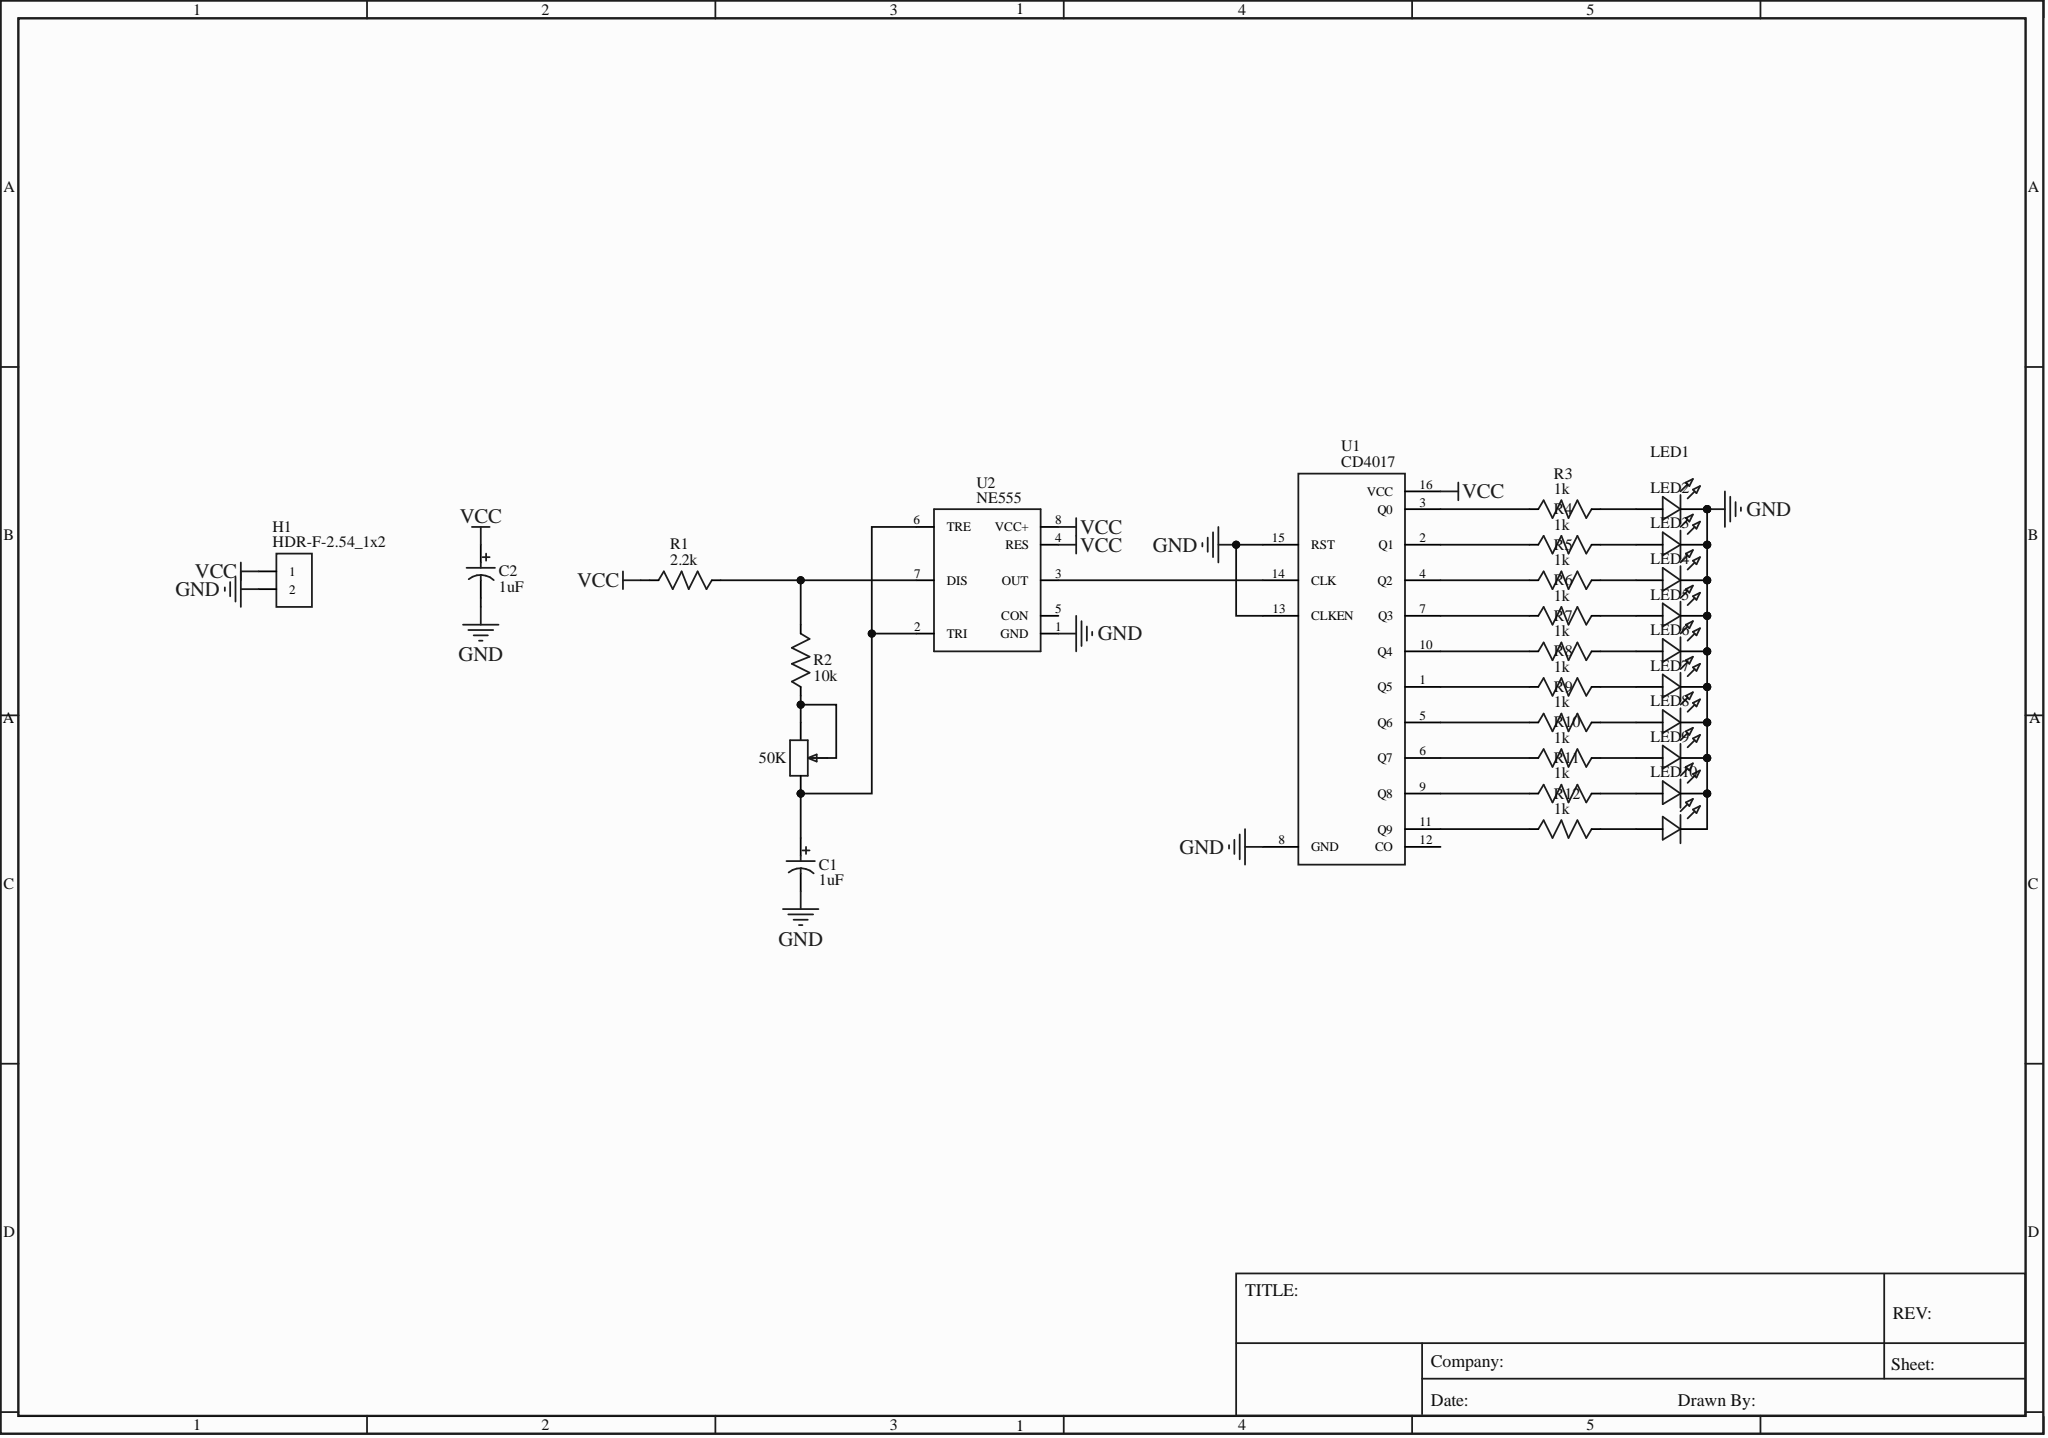Circuit board | Altium Designer | 28 parts | 26 nets
Bill of materials:
Comment,Description,Designator,Footprint,LibRef,Quantity
"1uF","","C1, C2","CAP-TH_BD5.0-P2.00-D0.8-FD","1uF 50V 5*11","2"
"HDR-F-2.54_1x2","","H1","HDR-F-2.54_1X2","HDR-F-2.54_1x2","1"
"LED-TH-3mm_R","","LED1, LED2, LED3, LED4, LED5, LED6, LED7, LED8, LED9, LED10","LED-TH_BD3.0_RED","204-10SDRD/S530-A3-L","10"
"2.2k","","R1","R_AXIAL-0.4","2.2k","1"
"10k","","R2","R_AXIAL-0.4","10k","1"
"1k","","R3, R4, R5, R6, R7, R8, R9, R10, R11, R12","R_AXIAL-0.4","1k","10"
"50K","","R13","RES-ADJ-SMD_RM065-V1","RM065-V1-5K blue","1"
"CD4017","","U1","CD4017","CD4017SOIC","1"
"NE555","","U2","DIP08-KIT","NE555","1"
Netlist (Protel format):
[
C1
CAP-TH_BD5.0-P2.00-D0.8-FD
1uF



]
[
C2
CAP-TH_BD5.0-P2.00-D0.8-FD
1uF



]
[
H1
HDR-F-2.54_1X2
HDR-F-2.54_1x2



]
[
LED1
LED-TH_BD3.0_RED
LED-TH-3mm_R



]
[
LED2
LED-TH_BD3.0_RED
LED-TH-3mm_R



]
[
LED3
LED-TH_BD3.0_RED
LED-TH-3mm_R



]
[
LED4
LED-TH_BD3.0_RED
LED-TH-3mm_R



]
[
LED5
LED-TH_BD3.0_RED
LED-TH-3mm_R



]
[
LED6
LED-TH_BD3.0_RED
LED-TH-3mm_R



]
[
LED7
LED-TH_BD3.0_RED
LED-TH-3mm_R



]
[
LED8
LED-TH_BD3.0_RED
LED-TH-3mm_R



]
[
LED9
LED-TH_BD3.0_RED
LED-TH-3mm_R



]
[
LED10
LED-TH_BD3.0_RED
LED-TH-3mm_R



]
[
R1
R_AXIAL-0.4
2.2k



]
[
R2
R_AXIAL-0.4
10k



]
[
R3
R_AXIAL-0.4
1k



]
[
R4
R_AXIAL-0.4
1k



]
[
R5
R_AXIAL-0.4
1k



]
[
R6
R_AXIAL-0.4
1k



]
[
R7
R_AXIAL-0.4
1k



]
[
R8
R_AXIAL-0.4
1k



]
[
R9
R_AXIAL-0.4
1k



]
[
R10
R_AXIAL-0.4
1k



]
[
R11
R_AXIAL-0.4
1k



]
[
R12
R_AXIAL-0.4
1k



]
[
R13
RES-ADJ-SMD_RM065-V1
50K



]
[
U1
CD4017
CD4017



]
[
U2
DIP08-KIT
NE555



]
(
VCC
C2-1
H1-1
R1-2
U1-16
U2-4
U2-8
)
(
NetU1_14
U1-14
U2-3
)
(
NetR12_1
R12-1
U1-11
)
(
NetR11_1
R11-1
U1-9
)
(
NetR10_1
R10-1
U1-6
)
(
NetR9_1
R9-1
U1-5
)
(
NetR8_1
R8-1
U1-1
)
(
NetR7_1
R7-1
U1-10
)
(
NetR6_1
R6-1
U1-7
)
(
NetR5_1
R5-1
U1-4
)
(
NetR4_1
R4-1
U1-2
)
(
NetR3_1
R3-1
U1-3
)
(
NetR2_1
R2-1
R13-1
R13-2
)
(
NetR1_1
R1-1
R2-2
U2-7
)
(
NetLED10_1
LED10-1
R12-2
)
(
NetLED9_1
LED9-1
R11-2
)
(
NetLED8_1
LED8-1
R10-2
)
(
NetLED7_1
LED7-1
R9-2
)
(
NetLED6_1
LED6-1
R8-2
)
(
NetLED5_1
LED5-1
R7-2
)
(
NetLED4_1
LED4-1
R6-2
)
(
NetLED3_1
LED3-1
R5-2
)
(
NetLED2_1
LED2-1
R4-2
)
(
NetLED1_1
LED1-1
R3-2
)
(
NetC1_1
C1-1
R13-3
U2-2
U2-6
)
(
GND
C1-2
C2-2
H1-2
LED1-2
LED2-2
LED3-2
LED4-2
LED5-2
LED6-2
LED7-2
LED8-2
LED9-2
LED10-2
U1-8
U1-13
U1-15
U2-1
)